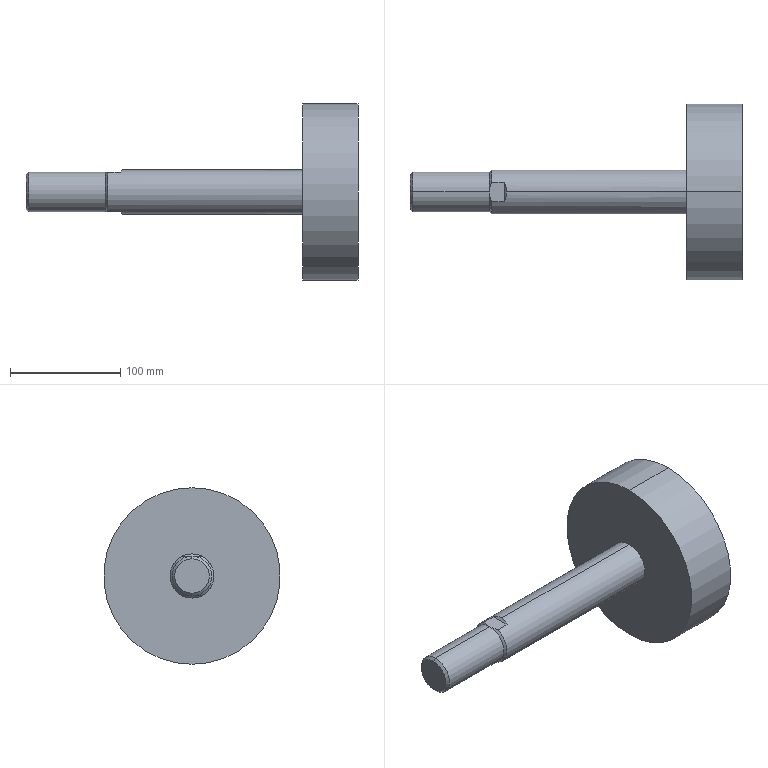Part | SolidWorks | features BaseBody 1 | 1 solid | 17 faces | box 301 x 160 x 160 mm | volume 1302352 mm3 | plane 7 | cylinder 6 | cone 4 | commonest cylinder face diameters 36 x2 40 x2 160 x2
STEP:
#1=CARTESIAN_POINT('',(138.,0.,-80.));
#2=VERTEX_POINT('',#1);
#3=CARTESIAN_POINT('',(138.,0.,80.));
#4=VERTEX_POINT('',#3);
#5=CARTESIAN_POINT('',(138.,0.,0.));
#6=DIRECTION('',(1.,0.,0.));
#7=DIRECTION('',(0.,0.,-1.));
#8=AXIS2_PLACEMENT_3D('',#5,#6,#7);
#9=CIRCLE('',#8,80.);
#10=EDGE_CURVE('',#2,#4,#9,.T.);
#11=ORIENTED_EDGE('',*,*,#10,.T.);
#12=CARTESIAN_POINT('',(188.,0.,80.));
#13=VERTEX_POINT('',#12);
#14=CARTESIAN_POINT('',(188.,0.,80.));
#15=DIRECTION('',(1.,0.,0.));
#16=VECTOR('',#15,1000.);
#17=LINE('',#14,#16);
#18=EDGE_CURVE('',#4,#13,#17,.T.);
#19=ORIENTED_EDGE('',*,*,#18,.T.);
#20=CARTESIAN_POINT('',(188.,0.,-80.));
#21=VERTEX_POINT('',#20);
#22=CARTESIAN_POINT('',(188.,0.,0.));
#23=DIRECTION('',(-1.,0.,0.));
#24=DIRECTION('',(0.,0.,-1.));
#25=AXIS2_PLACEMENT_3D('',#22,#23,#24);
#26=CIRCLE('',#25,80.);
#27=EDGE_CURVE('',#13,#21,#26,.T.);
#28=ORIENTED_EDGE('',*,*,#27,.T.);
#29=CARTESIAN_POINT('',(188.,0.,-80.));
#30=DIRECTION('',(1.,0.,0.));
#31=VECTOR('',#30,1000.);
#32=LINE('',#29,#31);
#33=EDGE_CURVE('',#2,#21,#32,.T.);
#34=ORIENTED_EDGE('',*,*,#33,.F.);
#35=EDGE_LOOP('',(#11,#19,#28,#34));
#36=FACE_OUTER_BOUND('',#35,.T.);
#37=CARTESIAN_POINT('',(188.,0.,0.));
#38=DIRECTION('',(1.,0.,0.));
#39=DIRECTION('',(0.,0.,-1.));
#40=AXIS2_PLACEMENT_3D('',#37,#38,#39);
#41=CYLINDRICAL_SURFACE('',#40,80.);
#42=ADVANCED_FACE('',(#36),#41,.T.);
#43=CARTESIAN_POINT('',(-27.5,8.718,18.));
#44=VERTEX_POINT('',#43);
#45=CARTESIAN_POINT('',(-25.5,0.,20.));
#46=VERTEX_POINT('',#45);
#47=CARTESIAN_POINT('',(-27.5,8.718,18.));
#48=CARTESIAN_POINT('',(-26.178,5.988,19.322));
#49=CARTESIAN_POINT('',(-25.5,3.033,20.));
#50=CARTESIAN_POINT('',(-25.5,0.,20.));
#51=(BOUNDED_CURVE()B_SPLINE_CURVE(3,(#47,#48,#49,#50),.UNSPECIFIED.,.F.,.F.)B_SPLINE_CURVE_WITH_KNOTS((4,4),(5.832,6.283),.UNSPECIFIED.)CURVE()GEOMETRIC_REPRESENTATION_ITEM()RATIONAL_B_SPLINE_CURVE((1.,0.9831,0.9831,1.))REPRESENTATION_ITEM(''));
#52=EDGE_CURVE('',#44,#46,#51,.T.);
#53=ORIENTED_EDGE('',*,*,#52,.T.);
#54=CARTESIAN_POINT('',(138.,0.,20.));
#55=VERTEX_POINT('',#54);
#56=CARTESIAN_POINT('',(188.,0.,20.));
#57=DIRECTION('',(1.,0.,0.));
#58=VECTOR('',#57,1000.);
#59=LINE('',#56,#58);
#60=EDGE_CURVE('',#46,#55,#59,.T.);
#61=ORIENTED_EDGE('',*,*,#60,.T.);
#62=CARTESIAN_POINT('',(138.,0.,-20.));
#63=VERTEX_POINT('',#62);
#64=CARTESIAN_POINT('',(138.,0.,0.));
#65=DIRECTION('',(-1.,0.,0.));
#66=DIRECTION('',(0.,0.,-1.));
#67=AXIS2_PLACEMENT_3D('',#64,#65,#66);
#68=CIRCLE('',#67,20.);
#69=EDGE_CURVE('',#55,#63,#68,.T.);
#70=ORIENTED_EDGE('',*,*,#69,.T.);
#71=CARTESIAN_POINT('',(-25.5,0.,-20.));
#72=VERTEX_POINT('',#71);
#73=CARTESIAN_POINT('',(188.,0.,-20.));
#74=DIRECTION('',(1.,0.,0.));
#75=VECTOR('',#74,1000.);
#76=LINE('',#73,#75);
#77=EDGE_CURVE('',#72,#63,#76,.T.);
#78=ORIENTED_EDGE('',*,*,#77,.F.);
#79=CARTESIAN_POINT('',(-27.5,8.718,-18.));
#80=VERTEX_POINT('',#79);
#81=CARTESIAN_POINT('',(-25.5,0.,-20.));
#82=CARTESIAN_POINT('',(-25.5,3.033,-20.));
#83=CARTESIAN_POINT('',(-26.178,5.988,-19.322));
#84=CARTESIAN_POINT('',(-27.5,8.718,-18.));
#85=(BOUNDED_CURVE()B_SPLINE_CURVE(3,(#81,#82,#83,#84),.UNSPECIFIED.,.F.,.F.)B_SPLINE_CURVE_WITH_KNOTS((4,4),(0.,0.451),.UNSPECIFIED.)CURVE()GEOMETRIC_REPRESENTATION_ITEM()RATIONAL_B_SPLINE_CURVE((1.,0.9831,0.9831,1.))REPRESENTATION_ITEM(''));
#86=EDGE_CURVE('',#72,#80,#85,.T.);
#87=ORIENTED_EDGE('',*,*,#86,.T.);
#88=CARTESIAN_POINT('',(-39.,8.718,-18.));
#89=VERTEX_POINT('',#88);
#90=CARTESIAN_POINT('',(188.,8.718,-18.));
#91=DIRECTION('',(-1.,0.,0.));
#92=VECTOR('',#91,1000.);
#93=LINE('',#90,#92);
#94=EDGE_CURVE('',#80,#89,#93,.T.);
#95=ORIENTED_EDGE('',*,*,#94,.T.);
#96=CARTESIAN_POINT('',(-39.,8.718,18.));
#97=VERTEX_POINT('',#96);
#98=CARTESIAN_POINT('',(-39.,0.,0.));
#99=DIRECTION('',(1.,0.,0.));
#100=DIRECTION('',(0.,0.,-1.));
#101=AXIS2_PLACEMENT_3D('',#98,#99,#100);
#102=CIRCLE('',#101,20.);
#103=EDGE_CURVE('',#89,#97,#102,.T.);
#104=ORIENTED_EDGE('',*,*,#103,.T.);
#105=CARTESIAN_POINT('',(188.,8.718,18.));
#106=DIRECTION('',(1.,0.,0.));
#107=VECTOR('',#106,1000.);
#108=LINE('',#105,#107);
#109=EDGE_CURVE('',#97,#44,#108,.T.);
#110=ORIENTED_EDGE('',*,*,#109,.T.);
#111=EDGE_LOOP('',(#53,#61,#70,#78,#87,#95,#104,#110));
#112=FACE_OUTER_BOUND('',#111,.T.);
#113=CARTESIAN_POINT('',(188.,0.,0.));
#114=DIRECTION('',(1.,0.,0.));
#115=DIRECTION('',(0.,0.,-1.));
#116=AXIS2_PLACEMENT_3D('',#113,#114,#115);
#117=CYLINDRICAL_SURFACE('',#116,20.);
#118=ADVANCED_FACE('',(#112),#117,.T.);
#119=CARTESIAN_POINT('',(-110.546,0.,-18.));
#120=VERTEX_POINT('',#119);
#121=CARTESIAN_POINT('',(-110.546,0.,18.));
#122=VERTEX_POINT('',#121);
#123=CARTESIAN_POINT('',(-110.546,0.,0.));
#124=DIRECTION('',(1.,0.,0.));
#125=DIRECTION('',(0.,0.,-1.));
#126=AXIS2_PLACEMENT_3D('',#123,#124,#125);
#127=CIRCLE('',#126,18.);
#128=EDGE_CURVE('',#120,#122,#127,.T.);
#129=ORIENTED_EDGE('',*,*,#128,.T.);
#130=CARTESIAN_POINT('',(-41.,0.,18.));
#131=VERTEX_POINT('',#130);
#132=CARTESIAN_POINT('',(188.,0.,18.));
#133=DIRECTION('',(1.,0.,0.));
#134=VECTOR('',#133,1000.);
#135=LINE('',#132,#134);
#136=EDGE_CURVE('',#122,#131,#135,.T.);
#137=ORIENTED_EDGE('',*,*,#136,.T.);
#138=CARTESIAN_POINT('',(-41.,0.,-18.));
#139=VERTEX_POINT('',#138);
#140=CARTESIAN_POINT('',(-41.,0.,0.));
#141=DIRECTION('',(1.,0.,0.));
#142=DIRECTION('',(0.,0.,-1.));
#143=AXIS2_PLACEMENT_3D('',#140,#141,#142);
#144=CIRCLE('',#143,18.);
#145=EDGE_CURVE('',#139,#131,#144,.T.);
#146=ORIENTED_EDGE('',*,*,#145,.F.);
#147=CARTESIAN_POINT('',(188.,0.,-18.));
#148=DIRECTION('',(1.,0.,0.));
#149=VECTOR('',#148,1000.);
#150=LINE('',#147,#149);
#151=EDGE_CURVE('',#120,#139,#150,.T.);
#152=ORIENTED_EDGE('',*,*,#151,.F.);
#153=EDGE_LOOP('',(#129,#137,#146,#152));
#154=FACE_OUTER_BOUND('',#153,.T.);
#155=CARTESIAN_POINT('',(188.,0.,0.));
#156=DIRECTION('',(1.,0.,0.));
#157=DIRECTION('',(0.,0.,-1.));
#158=AXIS2_PLACEMENT_3D('',#155,#156,#157);
#159=CYLINDRICAL_SURFACE('',#158,18.);
#160=ADVANCED_FACE('',(#154),#159,.T.);
#161=CARTESIAN_POINT('',(-113.,0.,-15.546));
#162=VERTEX_POINT('',#161);
#163=CARTESIAN_POINT('',(-113.,0.,15.546));
#164=VERTEX_POINT('',#163);
#165=CARTESIAN_POINT('',(-113.,0.,0.));
#166=DIRECTION('',(1.,0.,0.));
#167=DIRECTION('',(0.,0.,-1.));
#168=AXIS2_PLACEMENT_3D('',#165,#166,#167);
#169=CIRCLE('',#168,15.546);
#170=EDGE_CURVE('',#162,#164,#169,.T.);
#171=ORIENTED_EDGE('',*,*,#170,.T.);
#172=CARTESIAN_POINT('',(-110.546,0.,18.));
#173=DIRECTION('',(0.7071,0.,0.7071));
#174=VECTOR('',#173,1000.);
#175=LINE('',#172,#174);
#176=EDGE_CURVE('',#164,#122,#175,.T.);
#177=ORIENTED_EDGE('',*,*,#176,.T.);
#178=ORIENTED_EDGE('',*,*,#128,.F.);
#179=CARTESIAN_POINT('',(-110.546,0.,-18.));
#180=DIRECTION('',(0.7071,0.,-0.7071));
#181=VECTOR('',#180,1000.);
#182=LINE('',#179,#181);
#183=EDGE_CURVE('',#162,#120,#182,.T.);
#184=ORIENTED_EDGE('',*,*,#183,.F.);
#185=EDGE_LOOP('',(#171,#177,#178,#184));
#186=FACE_OUTER_BOUND('',#185,.T.);
#187=CARTESIAN_POINT('',(-110.546,0.,0.));
#188=DIRECTION('',(1.,0.,0.));
#189=DIRECTION('',(0.,0.,-1.));
#190=AXIS2_PLACEMENT_3D('',#187,#188,#189);
#191=CONICAL_SURFACE('',#190,18.,0.7854);
#192=ADVANCED_FACE('',(#186),#191,.T.);
#193=ORIENTED_EDGE('',*,*,#18,.F.);
#194=CARTESIAN_POINT('',(138.,0.,0.));
#195=DIRECTION('',(1.,0.,0.));
#196=DIRECTION('',(0.,0.,-1.));
#197=AXIS2_PLACEMENT_3D('',#194,#195,#196);
#198=CIRCLE('',#197,80.);
#199=EDGE_CURVE('',#4,#2,#198,.T.);
#200=ORIENTED_EDGE('',*,*,#199,.T.);
#201=ORIENTED_EDGE('',*,*,#33,.T.);
#202=CARTESIAN_POINT('',(188.,0.,0.));
#203=DIRECTION('',(-1.,0.,0.));
#204=DIRECTION('',(0.,0.,-1.));
#205=AXIS2_PLACEMENT_3D('',#202,#203,#204);
#206=CIRCLE('',#205,80.);
#207=EDGE_CURVE('',#21,#13,#206,.T.);
#208=ORIENTED_EDGE('',*,*,#207,.T.);
#209=EDGE_LOOP('',(#193,#200,#201,#208));
#210=FACE_OUTER_BOUND('',#209,.T.);
#211=CARTESIAN_POINT('',(188.,0.,0.));
#212=DIRECTION('',(1.,0.,0.));
#213=DIRECTION('',(0.,0.,-1.));
#214=AXIS2_PLACEMENT_3D('',#211,#212,#213);
#215=CYLINDRICAL_SURFACE('',#214,80.);
#216=ADVANCED_FACE('',(#210),#215,.T.);
#217=CARTESIAN_POINT('',(138.,0.,0.));
#218=DIRECTION('',(-1.,0.,0.));
#219=DIRECTION('',(0.,0.,-1.));
#220=AXIS2_PLACEMENT_3D('',#217,#218,#219);
#221=CIRCLE('',#220,20.);
#222=EDGE_CURVE('',#63,#55,#221,.T.);
#223=ORIENTED_EDGE('',*,*,#222,.F.);
#224=ORIENTED_EDGE('',*,*,#69,.F.);
#225=EDGE_LOOP('',(#223,#224));
#226=FACE_BOUND('',#225,.T.);
#227=ORIENTED_EDGE('',*,*,#10,.F.);
#228=ORIENTED_EDGE('',*,*,#199,.F.);
#229=EDGE_LOOP('',(#227,#228));
#230=FACE_OUTER_BOUND('',#229,.T.);
#231=CARTESIAN_POINT('',(138.,20.,0.));
#232=DIRECTION('',(1.,0.,0.));
#233=DIRECTION('',(0.,0.,-1.));
#234=AXIS2_PLACEMENT_3D('',#231,#232,#233);
#235=PLANE('',#234);
#236=ADVANCED_FACE('',(#226,#230),#235,.F.);
#237=ORIENTED_EDGE('',*,*,#207,.F.);
#238=ORIENTED_EDGE('',*,*,#27,.F.);
#239=EDGE_LOOP('',(#237,#238));
#240=FACE_OUTER_BOUND('',#239,.T.);
#241=CARTESIAN_POINT('',(188.,80.,0.));
#242=DIRECTION('',(-1.,0.,0.));
#243=DIRECTION('',(0.,0.,1.));
#244=AXIS2_PLACEMENT_3D('',#241,#242,#243);
#245=PLANE('',#244);
#246=ADVANCED_FACE('',(#240),#245,.F.);
#247=ORIENTED_EDGE('',*,*,#60,.F.);
#248=CARTESIAN_POINT('',(-27.5,-8.718,18.));
#249=VERTEX_POINT('',#248);
#250=CARTESIAN_POINT('',(-25.5,0.,20.));
#251=CARTESIAN_POINT('',(-25.5,-3.033,20.));
#252=CARTESIAN_POINT('',(-26.178,-5.988,19.322));
#253=CARTESIAN_POINT('',(-27.5,-8.718,18.));
#254=(BOUNDED_CURVE()B_SPLINE_CURVE(3,(#250,#251,#252,#253),.UNSPECIFIED.,.F.,.T.)B_SPLINE_CURVE_WITH_KNOTS((4,4),(0.,0.451),.UNSPECIFIED.)CURVE()GEOMETRIC_REPRESENTATION_ITEM()RATIONAL_B_SPLINE_CURVE((1.,0.9831,0.9831,1.))REPRESENTATION_ITEM(''));
#255=EDGE_CURVE('',#46,#249,#254,.T.);
#256=ORIENTED_EDGE('',*,*,#255,.T.);
#257=CARTESIAN_POINT('',(-39.,-8.718,18.));
#258=VERTEX_POINT('',#257);
#259=CARTESIAN_POINT('',(188.,-8.718,18.));
#260=DIRECTION('',(-1.,0.,0.));
#261=VECTOR('',#260,1000.);
#262=LINE('',#259,#261);
#263=EDGE_CURVE('',#249,#258,#262,.T.);
#264=ORIENTED_EDGE('',*,*,#263,.T.);
#265=CARTESIAN_POINT('',(-39.,-8.718,-18.));
#266=VERTEX_POINT('',#265);
#267=CARTESIAN_POINT('',(-39.,0.,0.));
#268=DIRECTION('',(1.,0.,0.));
#269=DIRECTION('',(0.,0.,-1.));
#270=AXIS2_PLACEMENT_3D('',#267,#268,#269);
#271=CIRCLE('',#270,20.);
#272=EDGE_CURVE('',#258,#266,#271,.T.);
#273=ORIENTED_EDGE('',*,*,#272,.T.);
#274=CARTESIAN_POINT('',(-27.5,-8.718,-18.));
#275=VERTEX_POINT('',#274);
#276=CARTESIAN_POINT('',(188.,-8.718,-18.));
#277=DIRECTION('',(1.,0.,0.));
#278=VECTOR('',#277,1000.);
#279=LINE('',#276,#278);
#280=EDGE_CURVE('',#266,#275,#279,.T.);
#281=ORIENTED_EDGE('',*,*,#280,.T.);
#282=CARTESIAN_POINT('',(-27.5,-8.718,-18.));
#283=CARTESIAN_POINT('',(-26.178,-5.988,-19.322));
#284=CARTESIAN_POINT('',(-25.5,-3.033,-20.));
#285=CARTESIAN_POINT('',(-25.5,0.,-20.));
#286=(BOUNDED_CURVE()B_SPLINE_CURVE(3,(#282,#283,#284,#285),.UNSPECIFIED.,.F.,.T.)B_SPLINE_CURVE_WITH_KNOTS((4,4),(5.832,6.283),.UNSPECIFIED.)CURVE()GEOMETRIC_REPRESENTATION_ITEM()RATIONAL_B_SPLINE_CURVE((1.,0.9831,0.9831,1.))REPRESENTATION_ITEM(''));
#287=EDGE_CURVE('',#275,#72,#286,.T.);
#288=ORIENTED_EDGE('',*,*,#287,.T.);
#289=ORIENTED_EDGE('',*,*,#77,.T.);
#290=ORIENTED_EDGE('',*,*,#222,.T.);
#291=EDGE_LOOP('',(#247,#256,#264,#273,#281,#288,#289,#290));
#292=FACE_OUTER_BOUND('',#291,.T.);
#293=CARTESIAN_POINT('',(188.,0.,0.));
#294=DIRECTION('',(1.,0.,0.));
#295=DIRECTION('',(0.,0.,-1.));
#296=AXIS2_PLACEMENT_3D('',#293,#294,#295);
#297=CYLINDRICAL_SURFACE('',#296,20.);
#298=ADVANCED_FACE('',(#292),#297,.T.);
#299=ORIENTED_EDGE('',*,*,#52,.F.);
#300=CARTESIAN_POINT('',(-27.5,20.,18.));
#301=DIRECTION('',(0.,-1.,0.));
#302=VECTOR('',#301,1000.);
#303=LINE('',#300,#302);
#304=EDGE_CURVE('',#44,#249,#303,.T.);
#305=ORIENTED_EDGE('',*,*,#304,.T.);
#306=ORIENTED_EDGE('',*,*,#255,.F.);
#307=EDGE_LOOP('',(#299,#305,#306));
#308=FACE_OUTER_BOUND('',#307,.T.);
#309=CARTESIAN_POINT('',(-25.5,20.,20.));
#310=DIRECTION('',(-0.7071,0.,0.7071));
#311=DIRECTION('',(0.7071,0.,0.7071));
#312=AXIS2_PLACEMENT_3D('',#309,#310,#311);
#313=PLANE('',#312);
#314=ADVANCED_FACE('',(#308),#313,.T.);
#315=CARTESIAN_POINT('',(-39.,8.718,18.));
#316=CARTESIAN_POINT('',(-39.603,7.335,18.));
#317=CARTESIAN_POINT('',(-40.102,5.925,18.));
#318=CARTESIAN_POINT('',(-40.627,3.748,18.));
#319=CARTESIAN_POINT('',(-40.765,3.012,18.));
#320=CARTESIAN_POINT('',(-40.951,1.517,18.));
#321=CARTESIAN_POINT('',(-41.,0.7578,18.));
#322=CARTESIAN_POINT('',(-41.,0.,18.));
#323=B_SPLINE_CURVE_WITH_KNOTS('',3,(#315,#316,#317,#318,#319,#320,#321,#322),.UNSPECIFIED.,.F.,.F.,(4,2,2,4),(0.,0.004476,0.006715,0.008953),.UNSPECIFIED.);
#324=EDGE_CURVE('',#97,#131,#323,.T.);
#325=ORIENTED_EDGE('',*,*,#324,.T.);
#326=CARTESIAN_POINT('',(-41.,0.,18.));
#327=CARTESIAN_POINT('',(-41.,-1.514,18.));
#328=CARTESIAN_POINT('',(-40.807,-2.995,18.));
#329=CARTESIAN_POINT('',(-40.284,-5.176,18.));
#330=CARTESIAN_POINT('',(-40.07,-5.897,18.));
#331=CARTESIAN_POINT('',(-39.578,-7.324,18.));
#332=CARTESIAN_POINT('',(-39.302,-8.026,18.));
#333=CARTESIAN_POINT('',(-39.,-8.718,18.));
#334=B_SPLINE_CURVE_WITH_KNOTS('',3,(#326,#327,#328,#329,#330,#331,#332,#333),.UNSPECIFIED.,.F.,.F.,(4,2,2,4),(0.,0.004476,0.006715,0.008953),.UNSPECIFIED.);
#335=EDGE_CURVE('',#131,#258,#334,.T.);
#336=ORIENTED_EDGE('',*,*,#335,.T.);
#337=ORIENTED_EDGE('',*,*,#263,.F.);
#338=ORIENTED_EDGE('',*,*,#304,.F.);
#339=ORIENTED_EDGE('',*,*,#109,.F.);
#340=EDGE_LOOP('',(#325,#336,#337,#338,#339));
#341=FACE_OUTER_BOUND('',#340,.T.);
#342=CARTESIAN_POINT('',(-27.5,20.,18.));
#343=DIRECTION('',(0.,0.,1.));
#344=DIRECTION('',(1.,0.,0.));
#345=AXIS2_PLACEMENT_3D('',#342,#343,#344);
#346=PLANE('',#345);
#347=ADVANCED_FACE('',(#341),#346,.T.);
#348=ORIENTED_EDGE('',*,*,#324,.F.);
#349=ORIENTED_EDGE('',*,*,#103,.F.);
#350=CARTESIAN_POINT('',(-39.,8.718,-18.));
#351=CARTESIAN_POINT('',(-39.603,7.335,-18.));
#352=CARTESIAN_POINT('',(-40.102,5.925,-18.));
#353=CARTESIAN_POINT('',(-40.627,3.748,-18.));
#354=CARTESIAN_POINT('',(-40.765,3.012,-18.));
#355=CARTESIAN_POINT('',(-40.951,1.517,-18.));
#356=CARTESIAN_POINT('',(-41.,0.7578,-18.));
#357=CARTESIAN_POINT('',(-41.,0.,-18.));
#358=B_SPLINE_CURVE_WITH_KNOTS('',3,(#350,#351,#352,#353,#354,#355,#356,#357),.UNSPECIFIED.,.F.,.F.,(4,2,2,4),(0.,0.004476,0.006715,0.008953),.UNSPECIFIED.);
#359=EDGE_CURVE('',#89,#139,#358,.T.);
#360=ORIENTED_EDGE('',*,*,#359,.T.);
#361=ORIENTED_EDGE('',*,*,#145,.T.);
#362=EDGE_LOOP('',(#348,#349,#360,#361));
#363=FACE_OUTER_BOUND('',#362,.T.);
#364=CARTESIAN_POINT('',(-39.,0.,0.));
#365=DIRECTION('',(1.,0.,0.));
#366=DIRECTION('',(0.,0.,-1.));
#367=AXIS2_PLACEMENT_3D('',#364,#365,#366);
#368=CONICAL_SURFACE('',#367,20.,0.7854);
#369=ADVANCED_FACE('',(#363),#368,.T.);
#370=CARTESIAN_POINT('',(-39.,-8.718,-18.));
#371=CARTESIAN_POINT('',(-39.603,-7.335,-18.));
#372=CARTESIAN_POINT('',(-40.102,-5.925,-18.));
#373=CARTESIAN_POINT('',(-40.627,-3.748,-18.));
#374=CARTESIAN_POINT('',(-40.765,-3.012,-18.));
#375=CARTESIAN_POINT('',(-40.951,-1.517,-18.));
#376=CARTESIAN_POINT('',(-41.,-0.7578,-18.));
#377=CARTESIAN_POINT('',(-41.,0.,-18.));
#378=B_SPLINE_CURVE_WITH_KNOTS('',3,(#370,#371,#372,#373,#374,#375,#376,#377),.UNSPECIFIED.,.F.,.F.,(4,2,2,4),(0.,0.004476,0.006715,0.008953),.UNSPECIFIED.);
#379=EDGE_CURVE('',#266,#139,#378,.T.);
#380=ORIENTED_EDGE('',*,*,#379,.T.);
#381=ORIENTED_EDGE('',*,*,#359,.F.);
#382=ORIENTED_EDGE('',*,*,#94,.F.);
#383=CARTESIAN_POINT('',(-27.5,20.,-18.));
#384=DIRECTION('',(0.,-1.,0.));
#385=VECTOR('',#384,1000.);
#386=LINE('',#383,#385);
#387=EDGE_CURVE('',#80,#275,#386,.T.);
#388=ORIENTED_EDGE('',*,*,#387,.T.);
#389=ORIENTED_EDGE('',*,*,#280,.F.);
#390=EDGE_LOOP('',(#380,#381,#382,#388,#389));
#391=FACE_OUTER_BOUND('',#390,.T.);
#392=CARTESIAN_POINT('',(-41.,20.,-18.));
#393=DIRECTION('',(0.,0.,-1.));
#394=DIRECTION('',(-1.,0.,0.));
#395=AXIS2_PLACEMENT_3D('',#392,#393,#394);
#396=PLANE('',#395);
#397=ADVANCED_FACE('',(#391),#396,.T.);
#398=ORIENTED_EDGE('',*,*,#287,.F.);
#399=ORIENTED_EDGE('',*,*,#387,.F.);
#400=ORIENTED_EDGE('',*,*,#86,.F.);
#401=EDGE_LOOP('',(#398,#399,#400));
#402=FACE_OUTER_BOUND('',#401,.T.);
#403=CARTESIAN_POINT('',(-27.5,20.,-18.));
#404=DIRECTION('',(-0.7071,0.,-0.7071));
#405=DIRECTION('',(-0.7071,0.,0.7071));
#406=AXIS2_PLACEMENT_3D('',#403,#404,#405);
#407=PLANE('',#406);
#408=ADVANCED_FACE('',(#402),#407,.T.);
#409=ORIENTED_EDGE('',*,*,#379,.F.);
#410=ORIENTED_EDGE('',*,*,#272,.F.);
#411=ORIENTED_EDGE('',*,*,#335,.F.);
#412=CARTESIAN_POINT('',(-41.,0.,0.));
#413=DIRECTION('',(1.,0.,0.));
#414=DIRECTION('',(0.,0.,-1.));
#415=AXIS2_PLACEMENT_3D('',#412,#413,#414);
#416=CIRCLE('',#415,18.);
#417=EDGE_CURVE('',#131,#139,#416,.T.);
#418=ORIENTED_EDGE('',*,*,#417,.T.);
#419=EDGE_LOOP('',(#409,#410,#411,#418));
#420=FACE_OUTER_BOUND('',#419,.T.);
#421=CARTESIAN_POINT('',(-39.,0.,0.));
#422=DIRECTION('',(1.,0.,0.));
#423=DIRECTION('',(0.,0.,-1.));
#424=AXIS2_PLACEMENT_3D('',#421,#422,#423);
#425=CONICAL_SURFACE('',#424,20.,0.7854);
#426=ADVANCED_FACE('',(#420),#425,.T.);
#427=ORIENTED_EDGE('',*,*,#136,.F.);
#428=CARTESIAN_POINT('',(-110.546,0.,0.));
#429=DIRECTION('',(1.,0.,0.));
#430=DIRECTION('',(0.,0.,-1.));
#431=AXIS2_PLACEMENT_3D('',#428,#429,#430);
#432=CIRCLE('',#431,18.);
#433=EDGE_CURVE('',#122,#120,#432,.T.);
#434=ORIENTED_EDGE('',*,*,#433,.T.);
#435=ORIENTED_EDGE('',*,*,#151,.T.);
#436=ORIENTED_EDGE('',*,*,#417,.F.);
#437=EDGE_LOOP('',(#427,#434,#435,#436));
#438=FACE_OUTER_BOUND('',#437,.T.);
#439=CARTESIAN_POINT('',(188.,0.,0.));
#440=DIRECTION('',(1.,0.,0.));
#441=DIRECTION('',(0.,0.,-1.));
#442=AXIS2_PLACEMENT_3D('',#439,#440,#441);
#443=CYLINDRICAL_SURFACE('',#442,18.);
#444=ADVANCED_FACE('',(#438),#443,.T.);
#445=ORIENTED_EDGE('',*,*,#176,.F.);
#446=CARTESIAN_POINT('',(-113.,0.,0.));
#447=DIRECTION('',(1.,0.,0.));
#448=DIRECTION('',(0.,0.,-1.));
#449=AXIS2_PLACEMENT_3D('',#446,#447,#448);
#450=CIRCLE('',#449,15.546);
#451=EDGE_CURVE('',#164,#162,#450,.T.);
#452=ORIENTED_EDGE('',*,*,#451,.T.);
#453=ORIENTED_EDGE('',*,*,#183,.T.);
#454=ORIENTED_EDGE('',*,*,#433,.F.);
#455=EDGE_LOOP('',(#445,#452,#453,#454));
#456=FACE_OUTER_BOUND('',#455,.T.);
#457=CARTESIAN_POINT('',(-110.546,0.,0.));
#458=DIRECTION('',(1.,0.,0.));
#459=DIRECTION('',(0.,0.,-1.));
#460=AXIS2_PLACEMENT_3D('',#457,#458,#459);
#461=CONICAL_SURFACE('',#460,18.,0.7854);
#462=ADVANCED_FACE('',(#456),#461,.T.);
#463=ORIENTED_EDGE('',*,*,#170,.F.);
#464=ORIENTED_EDGE('',*,*,#451,.F.);
#465=EDGE_LOOP('',(#463,#464));
#466=FACE_OUTER_BOUND('',#465,.T.);
#467=CARTESIAN_POINT('',(-113.,0.,0.));
#468=DIRECTION('',(1.,0.,0.));
#469=DIRECTION('',(0.,0.,-1.));
#470=AXIS2_PLACEMENT_3D('',#467,#468,#469);
#471=PLANE('',#470);
#472=ADVANCED_FACE('',(#466),#471,.F.);
#473=CLOSED_SHELL('',(#42,#118,#160,#192,#216,#236,#246,#298,#314,#347,#369,#397,#408,#426,#444,#462,#472));
#474=MANIFOLD_SOLID_BREP('',#473);
#475=CARTESIAN_POINT('',(0.,0.,0.));
#476=DIRECTION('',(0.,0.,1.));
#477=DIRECTION('',(1.,0.,0.));
#478=AXIS2_PLACEMENT_3D('',#475,#476,#477);
#479=(LENGTH_UNIT()NAMED_UNIT(*)SI_UNIT(.MILLI.,.METRE.));
#480=UNCERTAINTY_MEASURE_WITH_UNIT(LENGTH_MEASURE(0.00001),#479,'','');
#481=(NAMED_UNIT(*)PLANE_ANGLE_UNIT()SI_UNIT($,.RADIAN.));
#482=(NAMED_UNIT(*)SI_UNIT($,.STERADIAN.)SOLID_ANGLE_UNIT());
#483=(GEOMETRIC_REPRESENTATION_CONTEXT(3)GLOBAL_UNCERTAINTY_ASSIGNED_CONTEXT((#480))GLOBAL_UNIT_ASSIGNED_CONTEXT((#479,#481,#482))REPRESENTATION_CONTEXT('',''));
#484=ADVANCED_BREP_SHAPE_REPRESENTATION('',(#474,#478),#483);